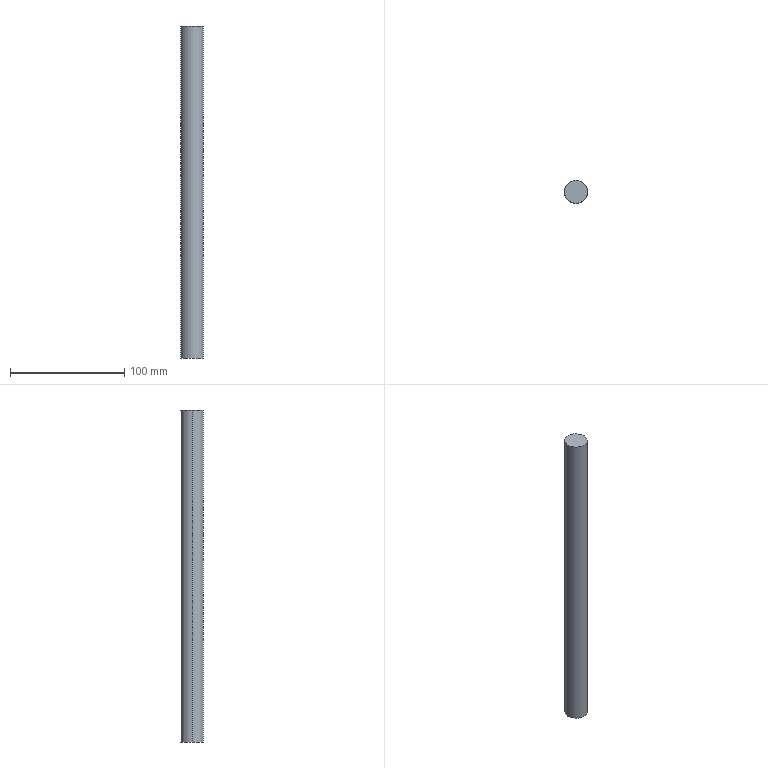Part | SolidWorks | features Extrusion 1 | 1 solid | 4 faces | box 20 x 20 x 290 mm | volume 91106 mm3 | cylinder 2 | plane 2 | commonest cylinder face diameters 20 x2
STEP:
#1=CARTESIAN_POINT('',(10.,0.,145.));
#2=VERTEX_POINT('',#1);
#3=CARTESIAN_POINT('',(-10.,0.,145.));
#4=VERTEX_POINT('',#3);
#5=CARTESIAN_POINT('',(0.,0.,145.));
#6=DIRECTION('',(0.,0.,1.));
#7=DIRECTION('',(1.,0.,0.));
#8=AXIS2_PLACEMENT_3D('',#5,#6,#7);
#9=CIRCLE('',#8,10.);
#10=EDGE_CURVE('',#2,#4,#9,.T.);
#11=ORIENTED_EDGE('',*,*,#10,.F.);
#12=CARTESIAN_POINT('',(10.,0.,-145.));
#13=VERTEX_POINT('',#12);
#14=CARTESIAN_POINT('',(10.,0.,145.));
#15=DIRECTION('',(0.,0.,-1.));
#16=VECTOR('',#15,1000.);
#17=LINE('',#14,#16);
#18=EDGE_CURVE('',#2,#13,#17,.T.);
#19=ORIENTED_EDGE('',*,*,#18,.T.);
#20=CARTESIAN_POINT('',(-10.,0.,-145.));
#21=VERTEX_POINT('',#20);
#22=CARTESIAN_POINT('',(0.,0.,-145.));
#23=DIRECTION('',(0.,0.,1.));
#24=DIRECTION('',(1.,0.,0.));
#25=AXIS2_PLACEMENT_3D('',#22,#23,#24);
#26=CIRCLE('',#25,10.);
#27=EDGE_CURVE('',#13,#21,#26,.T.);
#28=ORIENTED_EDGE('',*,*,#27,.T.);
#29=CARTESIAN_POINT('',(-10.,0.,145.));
#30=DIRECTION('',(0.,0.,-1.));
#31=VECTOR('',#30,1000.);
#32=LINE('',#29,#31);
#33=EDGE_CURVE('',#4,#21,#32,.T.);
#34=ORIENTED_EDGE('',*,*,#33,.F.);
#35=EDGE_LOOP('',(#11,#19,#28,#34));
#36=FACE_OUTER_BOUND('',#35,.T.);
#37=CARTESIAN_POINT('',(0.,0.,145.));
#38=DIRECTION('',(0.,0.,-1.));
#39=DIRECTION('',(-1.,0.,0.));
#40=AXIS2_PLACEMENT_3D('',#37,#38,#39);
#41=CYLINDRICAL_SURFACE('',#40,10.);
#42=ADVANCED_FACE('',(#36),#41,.T.);
#43=ORIENTED_EDGE('',*,*,#18,.F.);
#44=CARTESIAN_POINT('',(0.,0.,145.));
#45=DIRECTION('',(0.,0.,1.));
#46=DIRECTION('',(1.,0.,0.));
#47=AXIS2_PLACEMENT_3D('',#44,#45,#46);
#48=CIRCLE('',#47,10.);
#49=EDGE_CURVE('',#4,#2,#48,.T.);
#50=ORIENTED_EDGE('',*,*,#49,.F.);
#51=ORIENTED_EDGE('',*,*,#33,.T.);
#52=CARTESIAN_POINT('',(0.,0.,-145.));
#53=DIRECTION('',(0.,0.,1.));
#54=DIRECTION('',(1.,0.,0.));
#55=AXIS2_PLACEMENT_3D('',#52,#53,#54);
#56=CIRCLE('',#55,10.);
#57=EDGE_CURVE('',#21,#13,#56,.T.);
#58=ORIENTED_EDGE('',*,*,#57,.T.);
#59=EDGE_LOOP('',(#43,#50,#51,#58));
#60=FACE_OUTER_BOUND('',#59,.T.);
#61=CARTESIAN_POINT('',(0.,0.,145.));
#62=DIRECTION('',(0.,0.,-1.));
#63=DIRECTION('',(-1.,0.,0.));
#64=AXIS2_PLACEMENT_3D('',#61,#62,#63);
#65=CYLINDRICAL_SURFACE('',#64,10.);
#66=ADVANCED_FACE('',(#60),#65,.T.);
#67=ORIENTED_EDGE('',*,*,#49,.T.);
#68=ORIENTED_EDGE('',*,*,#10,.T.);
#69=EDGE_LOOP('',(#67,#68));
#70=FACE_OUTER_BOUND('',#69,.T.);
#71=CARTESIAN_POINT('',(0.,0.,145.));
#72=DIRECTION('',(0.,0.,1.));
#73=DIRECTION('',(1.,0.,0.));
#74=AXIS2_PLACEMENT_3D('',#71,#72,#73);
#75=PLANE('',#74);
#76=ADVANCED_FACE('',(#70),#75,.T.);
#77=ORIENTED_EDGE('',*,*,#57,.F.);
#78=ORIENTED_EDGE('',*,*,#27,.F.);
#79=EDGE_LOOP('',(#77,#78));
#80=FACE_OUTER_BOUND('',#79,.T.);
#81=CARTESIAN_POINT('',(0.,0.,-145.));
#82=DIRECTION('',(0.,0.,1.));
#83=DIRECTION('',(1.,0.,0.));
#84=AXIS2_PLACEMENT_3D('',#81,#82,#83);
#85=PLANE('',#84);
#86=ADVANCED_FACE('',(#80),#85,.F.);
#87=CLOSED_SHELL('',(#42,#66,#76,#86));
#88=MANIFOLD_SOLID_BREP('',#87);
#89=CARTESIAN_POINT('',(0.,0.,0.));
#90=DIRECTION('',(0.,0.,1.));
#91=DIRECTION('',(1.,0.,0.));
#92=AXIS2_PLACEMENT_3D('',#89,#90,#91);
#93=(LENGTH_UNIT()NAMED_UNIT(*)SI_UNIT(.MILLI.,.METRE.));
#94=UNCERTAINTY_MEASURE_WITH_UNIT(LENGTH_MEASURE(0.00001),#93,'','');
#95=(NAMED_UNIT(*)PLANE_ANGLE_UNIT()SI_UNIT($,.RADIAN.));
#96=(NAMED_UNIT(*)SI_UNIT($,.STERADIAN.)SOLID_ANGLE_UNIT());
#97=(GEOMETRIC_REPRESENTATION_CONTEXT(3)GLOBAL_UNCERTAINTY_ASSIGNED_CONTEXT((#94))GLOBAL_UNIT_ASSIGNED_CONTEXT((#93,#95,#96))REPRESENTATION_CONTEXT('',''));
#98=ADVANCED_BREP_SHAPE_REPRESENTATION('',(#88,#92),#97);